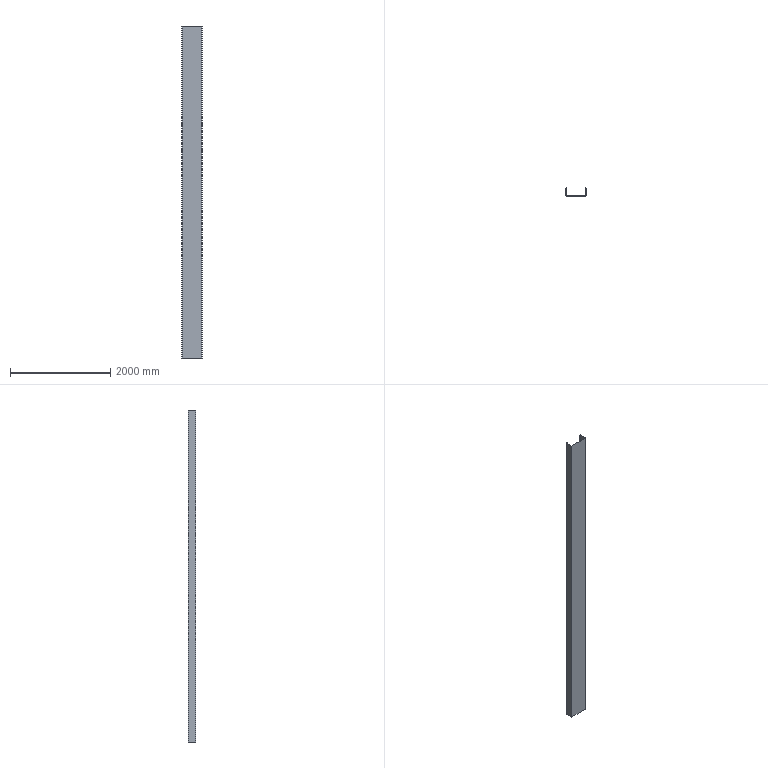Part | STEP file | 750038232 | 1 solid | 22 faces | box 400 x 150 x 6614 mm | volume 7243143 mm3 | plane 14 | cylinder 8 | commonest cylinder face diameters 3 x4 6 x4
STEP:
#1=CARTESIAN_POINT('',(-197.,0.,0.));
#2=VERTEX_POINT('',#1);
#3=CARTESIAN_POINT('',(-197.,0.,6613.5));
#4=VERTEX_POINT('',#3);
#5=CARTESIAN_POINT('',(-197.,0.,0.));
#6=DIRECTION('',(0.,0.,1.));
#7=VECTOR('',#6,1000.);
#8=LINE('',#5,#7);
#9=EDGE_CURVE('',#2,#4,#8,.T.);
#10=ORIENTED_EDGE('',*,*,#9,.F.);
#11=CARTESIAN_POINT('',(197.,0.,0.));
#12=VERTEX_POINT('',#11);
#13=CARTESIAN_POINT('',(200.,0.,0.));
#14=DIRECTION('',(-1.,0.,0.));
#15=VECTOR('',#14,1000.);
#16=LINE('',#13,#15);
#17=EDGE_CURVE('',#12,#2,#16,.T.);
#18=ORIENTED_EDGE('',*,*,#17,.F.);
#19=CARTESIAN_POINT('',(197.,0.,6613.5));
#20=VERTEX_POINT('',#19);
#21=CARTESIAN_POINT('',(197.,0.,0.));
#22=DIRECTION('',(0.,0.,-1.));
#23=VECTOR('',#22,1000.);
#24=LINE('',#21,#23);
#25=EDGE_CURVE('',#20,#12,#24,.T.);
#26=ORIENTED_EDGE('',*,*,#25,.F.);
#27=CARTESIAN_POINT('',(200.,0.,6613.5));
#28=DIRECTION('',(1.,0.,0.));
#29=VECTOR('',#28,1000.);
#30=LINE('',#27,#29);
#31=EDGE_CURVE('',#4,#20,#30,.T.);
#32=ORIENTED_EDGE('',*,*,#31,.F.);
#33=EDGE_LOOP('',(#10,#18,#26,#32));
#34=FACE_OUTER_BOUND('',#33,.T.);
#35=CARTESIAN_POINT('',(200.,0.,0.));
#36=DIRECTION('',(0.,1.,0.));
#37=DIRECTION('',(0.,0.,1.));
#38=AXIS2_PLACEMENT_3D('',#35,#36,#37);
#39=PLANE('',#38);
#40=ADVANCED_FACE('',(#34),#39,.F.);
#41=CARTESIAN_POINT('',(198.5,3.,6613.5));
#42=VERTEX_POINT('',#41);
#43=CARTESIAN_POINT('',(198.5,147.,6613.5));
#44=VERTEX_POINT('',#43);
#45=CARTESIAN_POINT('',(198.5,147.,6613.5));
#46=DIRECTION('',(0.,1.,0.));
#47=VECTOR('',#46,1000.);
#48=LINE('',#45,#47);
#49=EDGE_CURVE('',#42,#44,#48,.T.);
#50=ORIENTED_EDGE('',*,*,#49,.F.);
#51=CARTESIAN_POINT('',(197.,1.5,6613.5));
#52=VERTEX_POINT('',#51);
#53=CARTESIAN_POINT('',(197.,3.,6613.5));
#54=DIRECTION('',(0.,0.,1.));
#55=DIRECTION('',(1.,0.,0.));
#56=AXIS2_PLACEMENT_3D('',#53,#54,#55);
#57=CIRCLE('',#56,1.5);
#58=EDGE_CURVE('',#52,#42,#57,.T.);
#59=ORIENTED_EDGE('',*,*,#58,.F.);
#60=CARTESIAN_POINT('',(-197.,1.5,6613.5));
#61=VERTEX_POINT('',#60);
#62=CARTESIAN_POINT('',(197.,1.5,6613.5));
#63=DIRECTION('',(1.,0.,0.));
#64=VECTOR('',#63,1000.);
#65=LINE('',#62,#64);
#66=EDGE_CURVE('',#61,#52,#65,.T.);
#67=ORIENTED_EDGE('',*,*,#66,.F.);
#68=CARTESIAN_POINT('',(-198.5,3.,6613.5));
#69=VERTEX_POINT('',#68);
#70=CARTESIAN_POINT('',(-197.,3.,6613.5));
#71=DIRECTION('',(0.,0.,1.));
#72=DIRECTION('',(1.,0.,0.));
#73=AXIS2_PLACEMENT_3D('',#70,#71,#72);
#74=CIRCLE('',#73,1.5);
#75=EDGE_CURVE('',#69,#61,#74,.T.);
#76=ORIENTED_EDGE('',*,*,#75,.F.);
#77=CARTESIAN_POINT('',(-198.5,147.,6613.5));
#78=VERTEX_POINT('',#77);
#79=CARTESIAN_POINT('',(-198.5,147.,6613.5));
#80=DIRECTION('',(0.,-1.,0.));
#81=VECTOR('',#80,1000.);
#82=LINE('',#79,#81);
#83=EDGE_CURVE('',#78,#69,#82,.T.);
#84=ORIENTED_EDGE('',*,*,#83,.F.);
#85=CARTESIAN_POINT('',(-197.,148.5,6613.5));
#86=VERTEX_POINT('',#85);
#87=CARTESIAN_POINT('',(-197.,147.,6613.5));
#88=DIRECTION('',(0.,0.,1.));
#89=DIRECTION('',(1.,0.,0.));
#90=AXIS2_PLACEMENT_3D('',#87,#88,#89);
#91=CIRCLE('',#90,1.5);
#92=EDGE_CURVE('',#86,#78,#91,.T.);
#93=ORIENTED_EDGE('',*,*,#92,.F.);
#94=CARTESIAN_POINT('',(-180.,148.5,6613.5));
#95=VERTEX_POINT('',#94);
#96=CARTESIAN_POINT('',(197.,148.5,6613.5));
#97=DIRECTION('',(-1.,0.,0.));
#98=VECTOR('',#97,1000.);
#99=LINE('',#96,#98);
#100=EDGE_CURVE('',#95,#86,#99,.T.);
#101=ORIENTED_EDGE('',*,*,#100,.F.);
#102=CARTESIAN_POINT('',(-180.,150.,6613.5));
#103=VERTEX_POINT('',#102);
#104=CARTESIAN_POINT('',(-180.,150.,6613.5));
#105=DIRECTION('',(0.,-1.,0.));
#106=VECTOR('',#105,1000.);
#107=LINE('',#104,#106);
#108=EDGE_CURVE('',#103,#95,#107,.T.);
#109=ORIENTED_EDGE('',*,*,#108,.F.);
#110=CARTESIAN_POINT('',(-197.,150.,6613.5));
#111=VERTEX_POINT('',#110);
#112=CARTESIAN_POINT('',(197.,150.,6613.5));
#113=DIRECTION('',(1.,0.,0.));
#114=VECTOR('',#113,1000.);
#115=LINE('',#112,#114);
#116=EDGE_CURVE('',#111,#103,#115,.T.);
#117=ORIENTED_EDGE('',*,*,#116,.F.);
#118=CARTESIAN_POINT('',(-200.,147.,6613.5));
#119=VERTEX_POINT('',#118);
#120=CARTESIAN_POINT('',(-197.,147.,6613.5));
#121=DIRECTION('',(0.,0.,-1.));
#122=DIRECTION('',(1.,0.,0.));
#123=AXIS2_PLACEMENT_3D('',#120,#121,#122);
#124=CIRCLE('',#123,3.);
#125=EDGE_CURVE('',#119,#111,#124,.T.);
#126=ORIENTED_EDGE('',*,*,#125,.F.);
#127=CARTESIAN_POINT('',(-200.,3.,6613.5));
#128=VERTEX_POINT('',#127);
#129=CARTESIAN_POINT('',(-200.,147.,6613.5));
#130=DIRECTION('',(0.,1.,0.));
#131=VECTOR('',#130,1000.);
#132=LINE('',#129,#131);
#133=EDGE_CURVE('',#128,#119,#132,.T.);
#134=ORIENTED_EDGE('',*,*,#133,.F.);
#135=CARTESIAN_POINT('',(-197.,3.,6613.5));
#136=DIRECTION('',(0.,0.,-1.));
#137=DIRECTION('',(1.,0.,0.));
#138=AXIS2_PLACEMENT_3D('',#135,#136,#137);
#139=CIRCLE('',#138,3.);
#140=EDGE_CURVE('',#4,#128,#139,.T.);
#141=ORIENTED_EDGE('',*,*,#140,.F.);
#142=ORIENTED_EDGE('',*,*,#31,.T.);
#143=CARTESIAN_POINT('',(200.,3.,6613.5));
#144=VERTEX_POINT('',#143);
#145=CARTESIAN_POINT('',(197.,3.,6613.5));
#146=DIRECTION('',(0.,0.,-1.));
#147=DIRECTION('',(1.,0.,0.));
#148=AXIS2_PLACEMENT_3D('',#145,#146,#147);
#149=CIRCLE('',#148,3.);
#150=EDGE_CURVE('',#144,#20,#149,.T.);
#151=ORIENTED_EDGE('',*,*,#150,.F.);
#152=CARTESIAN_POINT('',(200.,147.,6613.5));
#153=VERTEX_POINT('',#152);
#154=CARTESIAN_POINT('',(200.,147.,6613.5));
#155=DIRECTION('',(0.,-1.,0.));
#156=VECTOR('',#155,1000.);
#157=LINE('',#154,#156);
#158=EDGE_CURVE('',#153,#144,#157,.T.);
#159=ORIENTED_EDGE('',*,*,#158,.F.);
#160=CARTESIAN_POINT('',(197.,150.,6613.5));
#161=VERTEX_POINT('',#160);
#162=CARTESIAN_POINT('',(197.,147.,6613.5));
#163=DIRECTION('',(0.,0.,-1.));
#164=DIRECTION('',(1.,0.,0.));
#165=AXIS2_PLACEMENT_3D('',#162,#163,#164);
#166=CIRCLE('',#165,3.);
#167=EDGE_CURVE('',#161,#153,#166,.T.);
#168=ORIENTED_EDGE('',*,*,#167,.F.);
#169=CARTESIAN_POINT('',(180.,150.,6613.5));
#170=VERTEX_POINT('',#169);
#171=CARTESIAN_POINT('',(197.,150.,6613.5));
#172=DIRECTION('',(1.,0.,0.));
#173=VECTOR('',#172,1000.);
#174=LINE('',#171,#173);
#175=EDGE_CURVE('',#170,#161,#174,.T.);
#176=ORIENTED_EDGE('',*,*,#175,.F.);
#177=CARTESIAN_POINT('',(180.,148.5,6613.5));
#178=VERTEX_POINT('',#177);
#179=CARTESIAN_POINT('',(180.,150.,6613.5));
#180=DIRECTION('',(0.,-1.,0.));
#181=VECTOR('',#180,1000.);
#182=LINE('',#179,#181);
#183=EDGE_CURVE('',#170,#178,#182,.T.);
#184=ORIENTED_EDGE('',*,*,#183,.T.);
#185=CARTESIAN_POINT('',(197.,148.5,6613.5));
#186=VERTEX_POINT('',#185);
#187=CARTESIAN_POINT('',(197.,148.5,6613.5));
#188=DIRECTION('',(-1.,0.,0.));
#189=VECTOR('',#188,1000.);
#190=LINE('',#187,#189);
#191=EDGE_CURVE('',#186,#178,#190,.T.);
#192=ORIENTED_EDGE('',*,*,#191,.F.);
#193=CARTESIAN_POINT('',(197.,147.,6613.5));
#194=DIRECTION('',(0.,0.,1.));
#195=DIRECTION('',(1.,0.,0.));
#196=AXIS2_PLACEMENT_3D('',#193,#194,#195);
#197=CIRCLE('',#196,1.5);
#198=EDGE_CURVE('',#44,#186,#197,.T.);
#199=ORIENTED_EDGE('',*,*,#198,.F.);
#200=EDGE_LOOP('',(#50,#59,#67,#76,#84,#93,#101,#109,#117,#126,#134,#141,#142,#151,#159,#168,#176,#184,#192,#199));
#201=FACE_OUTER_BOUND('',#200,.T.);
#202=CARTESIAN_POINT('',(197.,147.,6613.5));
#203=DIRECTION('',(0.,0.,-1.));
#204=DIRECTION('',(-1.,0.,0.));
#205=AXIS2_PLACEMENT_3D('',#202,#203,#204);
#206=PLANE('',#205);
#207=ADVANCED_FACE('',(#201),#206,.F.);
#208=CARTESIAN_POINT('',(-200.,3.,0.));
#209=VERTEX_POINT('',#208);
#210=CARTESIAN_POINT('',(-197.,3.,0.));
#211=DIRECTION('',(0.,0.,1.));
#212=DIRECTION('',(1.,0.,0.));
#213=AXIS2_PLACEMENT_3D('',#210,#211,#212);
#214=CIRCLE('',#213,3.);
#215=EDGE_CURVE('',#209,#2,#214,.T.);
#216=ORIENTED_EDGE('',*,*,#215,.T.);
#217=ORIENTED_EDGE('',*,*,#9,.T.);
#218=ORIENTED_EDGE('',*,*,#140,.T.);
#219=CARTESIAN_POINT('',(-200.,3.,0.));
#220=DIRECTION('',(0.,0.,-1.));
#221=VECTOR('',#220,1000.);
#222=LINE('',#219,#221);
#223=EDGE_CURVE('',#128,#209,#222,.T.);
#224=ORIENTED_EDGE('',*,*,#223,.T.);
#225=EDGE_LOOP('',(#216,#217,#218,#224));
#226=FACE_OUTER_BOUND('',#225,.T.);
#227=CARTESIAN_POINT('',(-197.,3.,0.));
#228=DIRECTION('',(0.,0.,1.));
#229=DIRECTION('',(1.,0.,0.));
#230=AXIS2_PLACEMENT_3D('',#227,#228,#229);
#231=CYLINDRICAL_SURFACE('',#230,3.);
#232=ADVANCED_FACE('',(#226),#231,.T.);
#233=CARTESIAN_POINT('',(197.,148.5,0.));
#234=VERTEX_POINT('',#233);
#235=CARTESIAN_POINT('',(180.,148.5,0.));
#236=VERTEX_POINT('',#235);
#237=CARTESIAN_POINT('',(180.,148.5,0.));
#238=DIRECTION('',(-1.,0.,0.));
#239=VECTOR('',#238,1000.);
#240=LINE('',#237,#239);
#241=EDGE_CURVE('',#234,#236,#240,.T.);
#242=ORIENTED_EDGE('',*,*,#241,.T.);
#243=CARTESIAN_POINT('',(180.,150.,0.));
#244=VERTEX_POINT('',#243);
#245=CARTESIAN_POINT('',(180.,150.,0.));
#246=DIRECTION('',(0.,1.,0.));
#247=VECTOR('',#246,1000.);
#248=LINE('',#245,#247);
#249=EDGE_CURVE('',#236,#244,#248,.T.);
#250=ORIENTED_EDGE('',*,*,#249,.T.);
#251=CARTESIAN_POINT('',(197.,150.,0.));
#252=VERTEX_POINT('',#251);
#253=CARTESIAN_POINT('',(180.,150.,0.));
#254=DIRECTION('',(1.,0.,0.));
#255=VECTOR('',#254,1000.);
#256=LINE('',#253,#255);
#257=EDGE_CURVE('',#244,#252,#256,.T.);
#258=ORIENTED_EDGE('',*,*,#257,.T.);
#259=CARTESIAN_POINT('',(200.,147.,0.));
#260=VERTEX_POINT('',#259);
#261=CARTESIAN_POINT('',(197.,147.,0.));
#262=DIRECTION('',(0.,0.,-1.));
#263=DIRECTION('',(1.,0.,0.));
#264=AXIS2_PLACEMENT_3D('',#261,#262,#263);
#265=CIRCLE('',#264,3.);
#266=EDGE_CURVE('',#252,#260,#265,.T.);
#267=ORIENTED_EDGE('',*,*,#266,.T.);
#268=CARTESIAN_POINT('',(200.,3.,0.));
#269=VERTEX_POINT('',#268);
#270=CARTESIAN_POINT('',(200.,150.,0.));
#271=DIRECTION('',(0.,-1.,0.));
#272=VECTOR('',#271,1000.);
#273=LINE('',#270,#272);
#274=EDGE_CURVE('',#260,#269,#273,.T.);
#275=ORIENTED_EDGE('',*,*,#274,.T.);
#276=CARTESIAN_POINT('',(197.,3.,0.));
#277=DIRECTION('',(0.,0.,-1.));
#278=DIRECTION('',(1.,0.,0.));
#279=AXIS2_PLACEMENT_3D('',#276,#277,#278);
#280=CIRCLE('',#279,3.);
#281=EDGE_CURVE('',#269,#12,#280,.T.);
#282=ORIENTED_EDGE('',*,*,#281,.T.);
#283=ORIENTED_EDGE('',*,*,#17,.T.);
#284=ORIENTED_EDGE('',*,*,#215,.F.);
#285=CARTESIAN_POINT('',(-200.,147.,0.));
#286=VERTEX_POINT('',#285);
#287=CARTESIAN_POINT('',(-200.,150.,0.));
#288=DIRECTION('',(0.,1.,0.));
#289=VECTOR('',#288,1000.);
#290=LINE('',#287,#289);
#291=EDGE_CURVE('',#209,#286,#290,.T.);
#292=ORIENTED_EDGE('',*,*,#291,.T.);
#293=CARTESIAN_POINT('',(-197.,150.,0.));
#294=VERTEX_POINT('',#293);
#295=CARTESIAN_POINT('',(-197.,147.,0.));
#296=DIRECTION('',(0.,0.,-1.));
#297=DIRECTION('',(1.,0.,0.));
#298=AXIS2_PLACEMENT_3D('',#295,#296,#297);
#299=CIRCLE('',#298,3.);
#300=EDGE_CURVE('',#286,#294,#299,.T.);
#301=ORIENTED_EDGE('',*,*,#300,.T.);
#302=CARTESIAN_POINT('',(-180.,150.,0.));
#303=VERTEX_POINT('',#302);
#304=CARTESIAN_POINT('',(180.,150.,0.));
#305=DIRECTION('',(1.,0.,0.));
#306=VECTOR('',#305,1000.);
#307=LINE('',#304,#306);
#308=EDGE_CURVE('',#294,#303,#307,.T.);
#309=ORIENTED_EDGE('',*,*,#308,.T.);
#310=CARTESIAN_POINT('',(-180.,148.5,0.));
#311=VERTEX_POINT('',#310);
#312=CARTESIAN_POINT('',(-180.,150.,0.));
#313=DIRECTION('',(0.,1.,0.));
#314=VECTOR('',#313,1000.);
#315=LINE('',#312,#314);
#316=EDGE_CURVE('',#311,#303,#315,.T.);
#317=ORIENTED_EDGE('',*,*,#316,.F.);
#318=CARTESIAN_POINT('',(-197.,148.5,0.));
#319=VERTEX_POINT('',#318);
#320=CARTESIAN_POINT('',(180.,148.5,0.));
#321=DIRECTION('',(-1.,0.,0.));
#322=VECTOR('',#321,1000.);
#323=LINE('',#320,#322);
#324=EDGE_CURVE('',#311,#319,#323,.T.);
#325=ORIENTED_EDGE('',*,*,#324,.T.);
#326=CARTESIAN_POINT('',(-198.5,147.,0.));
#327=VERTEX_POINT('',#326);
#328=CARTESIAN_POINT('',(-197.,147.,0.));
#329=DIRECTION('',(0.,0.,1.));
#330=DIRECTION('',(1.,0.,0.));
#331=AXIS2_PLACEMENT_3D('',#328,#329,#330);
#332=CIRCLE('',#331,1.5);
#333=EDGE_CURVE('',#319,#327,#332,.T.);
#334=ORIENTED_EDGE('',*,*,#333,.T.);
#335=CARTESIAN_POINT('',(-198.5,3.,0.));
#336=VERTEX_POINT('',#335);
#337=CARTESIAN_POINT('',(-198.5,150.,0.));
#338=DIRECTION('',(0.,-1.,0.));
#339=VECTOR('',#338,1000.);
#340=LINE('',#337,#339);
#341=EDGE_CURVE('',#327,#336,#340,.T.);
#342=ORIENTED_EDGE('',*,*,#341,.T.);
#343=CARTESIAN_POINT('',(-197.,1.5,0.));
#344=VERTEX_POINT('',#343);
#345=CARTESIAN_POINT('',(-197.,3.,0.));
#346=DIRECTION('',(0.,0.,1.));
#347=DIRECTION('',(1.,0.,0.));
#348=AXIS2_PLACEMENT_3D('',#345,#346,#347);
#349=CIRCLE('',#348,1.5);
#350=EDGE_CURVE('',#336,#344,#349,.T.);
#351=ORIENTED_EDGE('',*,*,#350,.T.);
#352=CARTESIAN_POINT('',(197.,1.5,0.));
#353=VERTEX_POINT('',#352);
#354=CARTESIAN_POINT('',(180.,1.5,0.));
#355=DIRECTION('',(1.,0.,0.));
#356=VECTOR('',#355,1000.);
#357=LINE('',#354,#356);
#358=EDGE_CURVE('',#344,#353,#357,.T.);
#359=ORIENTED_EDGE('',*,*,#358,.T.);
#360=CARTESIAN_POINT('',(198.5,3.,0.));
#361=VERTEX_POINT('',#360);
#362=CARTESIAN_POINT('',(197.,3.,0.));
#363=DIRECTION('',(0.,0.,1.));
#364=DIRECTION('',(1.,0.,0.));
#365=AXIS2_PLACEMENT_3D('',#362,#363,#364);
#366=CIRCLE('',#365,1.5);
#367=EDGE_CURVE('',#353,#361,#366,.T.);
#368=ORIENTED_EDGE('',*,*,#367,.T.);
#369=CARTESIAN_POINT('',(198.5,147.,0.));
#370=VERTEX_POINT('',#369);
#371=CARTESIAN_POINT('',(198.5,150.,0.));
#372=DIRECTION('',(0.,1.,0.));
#373=VECTOR('',#372,1000.);
#374=LINE('',#371,#373);
#375=EDGE_CURVE('',#361,#370,#374,.T.);
#376=ORIENTED_EDGE('',*,*,#375,.T.);
#377=CARTESIAN_POINT('',(197.,147.,0.));
#378=DIRECTION('',(0.,0.,1.));
#379=DIRECTION('',(1.,0.,0.));
#380=AXIS2_PLACEMENT_3D('',#377,#378,#379);
#381=CIRCLE('',#380,1.5);
#382=EDGE_CURVE('',#370,#234,#381,.T.);
#383=ORIENTED_EDGE('',*,*,#382,.T.);
#384=EDGE_LOOP('',(#242,#250,#258,#267,#275,#282,#283,#284,#292,#301,#309,#317,#325,#334,#342,#351,#359,#368,#376,#383));
#385=FACE_OUTER_BOUND('',#384,.T.);
#386=CARTESIAN_POINT('',(180.,150.,0.));
#387=DIRECTION('',(0.,0.,-1.));
#388=DIRECTION('',(-1.,0.,0.));
#389=AXIS2_PLACEMENT_3D('',#386,#387,#388);
#390=PLANE('',#389);
#391=ADVANCED_FACE('',(#385),#390,.T.);
#392=ORIENTED_EDGE('',*,*,#281,.F.);
#393=CARTESIAN_POINT('',(200.,3.,0.));
#394=DIRECTION('',(0.,0.,1.));
#395=VECTOR('',#394,1000.);
#396=LINE('',#393,#395);
#397=EDGE_CURVE('',#269,#144,#396,.T.);
#398=ORIENTED_EDGE('',*,*,#397,.T.);
#399=ORIENTED_EDGE('',*,*,#150,.T.);
#400=ORIENTED_EDGE('',*,*,#25,.T.);
#401=EDGE_LOOP('',(#392,#398,#399,#400));
#402=FACE_OUTER_BOUND('',#401,.T.);
#403=CARTESIAN_POINT('',(197.,3.,0.));
#404=DIRECTION('',(0.,0.,1.));
#405=DIRECTION('',(1.,0.,0.));
#406=AXIS2_PLACEMENT_3D('',#403,#404,#405);
#407=CYLINDRICAL_SURFACE('',#406,3.);
#408=ADVANCED_FACE('',(#402),#407,.T.);
#409=CARTESIAN_POINT('',(197.,148.5,0.));
#410=DIRECTION('',(0.,0.,1.));
#411=VECTOR('',#410,1000.);
#412=LINE('',#409,#411);
#413=EDGE_CURVE('',#234,#186,#412,.T.);
#414=ORIENTED_EDGE('',*,*,#413,.F.);
#415=ORIENTED_EDGE('',*,*,#382,.F.);
#416=CARTESIAN_POINT('',(198.5,147.,0.));
#417=DIRECTION('',(0.,0.,-1.));
#418=VECTOR('',#417,1000.);
#419=LINE('',#416,#418);
#420=EDGE_CURVE('',#44,#370,#419,.T.);
#421=ORIENTED_EDGE('',*,*,#420,.F.);
#422=ORIENTED_EDGE('',*,*,#198,.T.);
#423=EDGE_LOOP('',(#414,#415,#421,#422));
#424=FACE_OUTER_BOUND('',#423,.T.);
#425=CARTESIAN_POINT('',(197.,147.,0.));
#426=DIRECTION('',(0.,0.,1.));
#427=DIRECTION('',(1.,0.,0.));
#428=AXIS2_PLACEMENT_3D('',#425,#426,#427);
#429=CYLINDRICAL_SURFACE('',#428,1.5);
#430=ADVANCED_FACE('',(#424),#429,.F.);
#431=ORIENTED_EDGE('',*,*,#375,.F.);
#432=CARTESIAN_POINT('',(198.5,3.,0.));
#433=DIRECTION('',(0.,0.,1.));
#434=VECTOR('',#433,1000.);
#435=LINE('',#432,#434);
#436=EDGE_CURVE('',#361,#42,#435,.T.);
#437=ORIENTED_EDGE('',*,*,#436,.T.);
#438=ORIENTED_EDGE('',*,*,#49,.T.);
#439=ORIENTED_EDGE('',*,*,#420,.T.);
#440=EDGE_LOOP('',(#431,#437,#438,#439));
#441=FACE_OUTER_BOUND('',#440,.T.);
#442=CARTESIAN_POINT('',(198.5,150.,0.));
#443=DIRECTION('',(-1.,0.,0.));
#444=DIRECTION('',(0.,0.,1.));
#445=AXIS2_PLACEMENT_3D('',#442,#443,#444);
#446=PLANE('',#445);
#447=ADVANCED_FACE('',(#441),#446,.T.);
#448=ORIENTED_EDGE('',*,*,#436,.F.);
#449=ORIENTED_EDGE('',*,*,#367,.F.);
#450=CARTESIAN_POINT('',(197.,1.5,0.));
#451=DIRECTION('',(0.,0.,-1.));
#452=VECTOR('',#451,1000.);
#453=LINE('',#450,#452);
#454=EDGE_CURVE('',#52,#353,#453,.T.);
#455=ORIENTED_EDGE('',*,*,#454,.F.);
#456=ORIENTED_EDGE('',*,*,#58,.T.);
#457=EDGE_LOOP('',(#448,#449,#455,#456));
#458=FACE_OUTER_BOUND('',#457,.T.);
#459=CARTESIAN_POINT('',(197.,3.,0.));
#460=DIRECTION('',(0.,0.,1.));
#461=DIRECTION('',(1.,0.,0.));
#462=AXIS2_PLACEMENT_3D('',#459,#460,#461);
#463=CYLINDRICAL_SURFACE('',#462,1.5);
#464=ADVANCED_FACE('',(#458),#463,.F.);
#465=ORIENTED_EDGE('',*,*,#358,.F.);
#466=CARTESIAN_POINT('',(-197.,1.5,0.));
#467=DIRECTION('',(0.,0.,1.));
#468=VECTOR('',#467,1000.);
#469=LINE('',#466,#468);
#470=EDGE_CURVE('',#344,#61,#469,.T.);
#471=ORIENTED_EDGE('',*,*,#470,.T.);
#472=ORIENTED_EDGE('',*,*,#66,.T.);
#473=ORIENTED_EDGE('',*,*,#454,.T.);
#474=EDGE_LOOP('',(#465,#471,#472,#473));
#475=FACE_OUTER_BOUND('',#474,.T.);
#476=CARTESIAN_POINT('',(200.,1.5,0.));
#477=DIRECTION('',(0.,1.,0.));
#478=DIRECTION('',(0.,0.,1.));
#479=AXIS2_PLACEMENT_3D('',#476,#477,#478);
#480=PLANE('',#479);
#481=ADVANCED_FACE('',(#475),#480,.T.);
#482=ORIENTED_EDGE('',*,*,#470,.F.);
#483=ORIENTED_EDGE('',*,*,#350,.F.);
#484=CARTESIAN_POINT('',(-198.5,3.,0.));
#485=DIRECTION('',(0.,0.,-1.));
#486=VECTOR('',#485,1000.);
#487=LINE('',#484,#486);
#488=EDGE_CURVE('',#69,#336,#487,.T.);
#489=ORIENTED_EDGE('',*,*,#488,.F.);
#490=ORIENTED_EDGE('',*,*,#75,.T.);
#491=EDGE_LOOP('',(#482,#483,#489,#490));
#492=FACE_OUTER_BOUND('',#491,.T.);
#493=CARTESIAN_POINT('',(-197.,3.,0.));
#494=DIRECTION('',(0.,0.,1.));
#495=DIRECTION('',(1.,0.,0.));
#496=AXIS2_PLACEMENT_3D('',#493,#494,#495);
#497=CYLINDRICAL_SURFACE('',#496,1.5);
#498=ADVANCED_FACE('',(#492),#497,.F.);
#499=ORIENTED_EDGE('',*,*,#341,.F.);
#500=CARTESIAN_POINT('',(-198.5,147.,0.));
#501=DIRECTION('',(0.,0.,1.));
#502=VECTOR('',#501,1000.);
#503=LINE('',#500,#502);
#504=EDGE_CURVE('',#327,#78,#503,.T.);
#505=ORIENTED_EDGE('',*,*,#504,.T.);
#506=ORIENTED_EDGE('',*,*,#83,.T.);
#507=ORIENTED_EDGE('',*,*,#488,.T.);
#508=EDGE_LOOP('',(#499,#505,#506,#507));
#509=FACE_OUTER_BOUND('',#508,.T.);
#510=CARTESIAN_POINT('',(-198.5,0.,0.));
#511=DIRECTION('',(1.,0.,0.));
#512=DIRECTION('',(0.,0.,-1.));
#513=AXIS2_PLACEMENT_3D('',#510,#511,#512);
#514=PLANE('',#513);
#515=ADVANCED_FACE('',(#509),#514,.T.);
#516=ORIENTED_EDGE('',*,*,#504,.F.);
#517=ORIENTED_EDGE('',*,*,#333,.F.);
#518=CARTESIAN_POINT('',(-197.,148.5,0.));
#519=DIRECTION('',(0.,0.,-1.));
#520=VECTOR('',#519,1000.);
#521=LINE('',#518,#520);
#522=EDGE_CURVE('',#86,#319,#521,.T.);
#523=ORIENTED_EDGE('',*,*,#522,.F.);
#524=ORIENTED_EDGE('',*,*,#92,.T.);
#525=EDGE_LOOP('',(#516,#517,#523,#524));
#526=FACE_OUTER_BOUND('',#525,.T.);
#527=CARTESIAN_POINT('',(-197.,147.,0.));
#528=DIRECTION('',(0.,0.,1.));
#529=DIRECTION('',(1.,0.,0.));
#530=AXIS2_PLACEMENT_3D('',#527,#528,#529);
#531=CYLINDRICAL_SURFACE('',#530,1.5);
#532=ADVANCED_FACE('',(#526),#531,.F.);
#533=ORIENTED_EDGE('',*,*,#324,.F.);
#534=CARTESIAN_POINT('',(-180.,148.5,0.));
#535=DIRECTION('',(0.,0.,1.));
#536=VECTOR('',#535,1000.);
#537=LINE('',#534,#536);
#538=EDGE_CURVE('',#311,#95,#537,.T.);
#539=ORIENTED_EDGE('',*,*,#538,.T.);
#540=ORIENTED_EDGE('',*,*,#100,.T.);
#541=ORIENTED_EDGE('',*,*,#522,.T.);
#542=EDGE_LOOP('',(#533,#539,#540,#541));
#543=FACE_OUTER_BOUND('',#542,.T.);
#544=CARTESIAN_POINT('',(-200.,148.5,0.));
#545=DIRECTION('',(0.,-1.,0.));
#546=DIRECTION('',(0.,0.,-1.));
#547=AXIS2_PLACEMENT_3D('',#544,#545,#546);
#548=PLANE('',#547);
#549=ADVANCED_FACE('',(#543),#548,.T.);
#550=CARTESIAN_POINT('',(-180.,150.,0.));
#551=DIRECTION('',(0.,0.,1.));
#552=VECTOR('',#551,1000.);
#553=LINE('',#550,#552);
#554=EDGE_CURVE('',#303,#103,#553,.T.);
#555=ORIENTED_EDGE('',*,*,#554,.F.);
#556=ORIENTED_EDGE('',*,*,#308,.F.);
#557=CARTESIAN_POINT('',(-197.,150.,0.));
#558=DIRECTION('',(0.,0.,-1.));
#559=VECTOR('',#558,1000.);
#560=LINE('',#557,#559);
#561=EDGE_CURVE('',#111,#294,#560,.T.);
#562=ORIENTED_EDGE('',*,*,#561,.F.);
#563=ORIENTED_EDGE('',*,*,#116,.T.);
#564=EDGE_LOOP('',(#555,#556,#562,#563));
#565=FACE_OUTER_BOUND('',#564,.T.);
#566=CARTESIAN_POINT('',(-200.,150.,0.));
#567=DIRECTION('',(0.,-1.,0.));
#568=DIRECTION('',(0.,0.,-1.));
#569=AXIS2_PLACEMENT_3D('',#566,#567,#568);
#570=PLANE('',#569);
#571=ADVANCED_FACE('',(#565),#570,.F.);
#572=ORIENTED_EDGE('',*,*,#300,.F.);
#573=CARTESIAN_POINT('',(-200.,147.,0.));
#574=DIRECTION('',(0.,0.,1.));
#575=VECTOR('',#574,1000.);
#576=LINE('',#573,#575);
#577=EDGE_CURVE('',#286,#119,#576,.T.);
#578=ORIENTED_EDGE('',*,*,#577,.T.);
#579=ORIENTED_EDGE('',*,*,#125,.T.);
#580=ORIENTED_EDGE('',*,*,#561,.T.);
#581=EDGE_LOOP('',(#572,#578,#579,#580));
#582=FACE_OUTER_BOUND('',#581,.T.);
#583=CARTESIAN_POINT('',(-197.,147.,0.));
#584=DIRECTION('',(0.,0.,1.));
#585=DIRECTION('',(1.,0.,0.));
#586=AXIS2_PLACEMENT_3D('',#583,#584,#585);
#587=CYLINDRICAL_SURFACE('',#586,3.);
#588=ADVANCED_FACE('',(#582),#587,.T.);
#589=ORIENTED_EDGE('',*,*,#577,.F.);
#590=ORIENTED_EDGE('',*,*,#291,.F.);
#591=ORIENTED_EDGE('',*,*,#223,.F.);
#592=ORIENTED_EDGE('',*,*,#133,.T.);
#593=EDGE_LOOP('',(#589,#590,#591,#592));
#594=FACE_OUTER_BOUND('',#593,.T.);
#595=CARTESIAN_POINT('',(-200.,0.,0.));
#596=DIRECTION('',(1.,0.,0.));
#597=DIRECTION('',(0.,0.,-1.));
#598=AXIS2_PLACEMENT_3D('',#595,#596,#597);
#599=PLANE('',#598);
#600=ADVANCED_FACE('',(#594),#599,.F.);
#601=ORIENTED_EDGE('',*,*,#397,.F.);
#602=ORIENTED_EDGE('',*,*,#274,.F.);
#603=CARTESIAN_POINT('',(200.,147.,0.));
#604=DIRECTION('',(0.,0.,-1.));
#605=VECTOR('',#604,1000.);
#606=LINE('',#603,#605);
#607=EDGE_CURVE('',#153,#260,#606,.T.);
#608=ORIENTED_EDGE('',*,*,#607,.F.);
#609=ORIENTED_EDGE('',*,*,#158,.T.);
#610=EDGE_LOOP('',(#601,#602,#608,#609));
#611=FACE_OUTER_BOUND('',#610,.T.);
#612=CARTESIAN_POINT('',(200.,150.,0.));
#613=DIRECTION('',(-1.,0.,0.));
#614=DIRECTION('',(0.,0.,1.));
#615=AXIS2_PLACEMENT_3D('',#612,#613,#614);
#616=PLANE('',#615);
#617=ADVANCED_FACE('',(#611),#616,.F.);
#618=ORIENTED_EDGE('',*,*,#266,.F.);
#619=CARTESIAN_POINT('',(197.,150.,0.));
#620=DIRECTION('',(0.,0.,1.));
#621=VECTOR('',#620,1000.);
#622=LINE('',#619,#621);
#623=EDGE_CURVE('',#252,#161,#622,.T.);
#624=ORIENTED_EDGE('',*,*,#623,.T.);
#625=ORIENTED_EDGE('',*,*,#167,.T.);
#626=ORIENTED_EDGE('',*,*,#607,.T.);
#627=EDGE_LOOP('',(#618,#624,#625,#626));
#628=FACE_OUTER_BOUND('',#627,.T.);
#629=CARTESIAN_POINT('',(197.,147.,0.));
#630=DIRECTION('',(0.,0.,1.));
#631=DIRECTION('',(1.,0.,0.));
#632=AXIS2_PLACEMENT_3D('',#629,#630,#631);
#633=CYLINDRICAL_SURFACE('',#632,3.);
#634=ADVANCED_FACE('',(#628),#633,.T.);
#635=ORIENTED_EDGE('',*,*,#623,.F.);
#636=ORIENTED_EDGE('',*,*,#257,.F.);
#637=CARTESIAN_POINT('',(180.,150.,0.));
#638=DIRECTION('',(0.,0.,-1.));
#639=VECTOR('',#638,1000.);
#640=LINE('',#637,#639);
#641=EDGE_CURVE('',#170,#244,#640,.T.);
#642=ORIENTED_EDGE('',*,*,#641,.F.);
#643=ORIENTED_EDGE('',*,*,#175,.T.);
#644=EDGE_LOOP('',(#635,#636,#642,#643));
#645=FACE_OUTER_BOUND('',#644,.T.);
#646=CARTESIAN_POINT('',(180.,150.,0.));
#647=DIRECTION('',(0.,-1.,0.));
#648=DIRECTION('',(0.,0.,-1.));
#649=AXIS2_PLACEMENT_3D('',#646,#647,#648);
#650=PLANE('',#649);
#651=ADVANCED_FACE('',(#645),#650,.F.);
#652=ORIENTED_EDGE('',*,*,#241,.F.);
#653=ORIENTED_EDGE('',*,*,#413,.T.);
#654=ORIENTED_EDGE('',*,*,#191,.T.);
#655=CARTESIAN_POINT('',(180.,148.5,0.));
#656=DIRECTION('',(0.,0.,-1.));
#657=VECTOR('',#656,1000.);
#658=LINE('',#655,#657);
#659=EDGE_CURVE('',#178,#236,#658,.T.);
#660=ORIENTED_EDGE('',*,*,#659,.T.);
#661=EDGE_LOOP('',(#652,#653,#654,#660));
#662=FACE_OUTER_BOUND('',#661,.T.);
#663=CARTESIAN_POINT('',(180.,148.5,0.));
#664=DIRECTION('',(0.,-1.,0.));
#665=DIRECTION('',(0.,0.,-1.));
#666=AXIS2_PLACEMENT_3D('',#663,#664,#665);
#667=PLANE('',#666);
#668=ADVANCED_FACE('',(#662),#667,.T.);
#669=ORIENTED_EDGE('',*,*,#316,.T.);
#670=ORIENTED_EDGE('',*,*,#554,.T.);
#671=ORIENTED_EDGE('',*,*,#108,.T.);
#672=ORIENTED_EDGE('',*,*,#538,.F.);
#673=EDGE_LOOP('',(#669,#670,#671,#672));
#674=FACE_OUTER_BOUND('',#673,.T.);
#675=CARTESIAN_POINT('',(-180.,150.,0.));
#676=DIRECTION('',(1.,0.,0.));
#677=DIRECTION('',(0.,0.,-1.));
#678=AXIS2_PLACEMENT_3D('',#675,#676,#677);
#679=PLANE('',#678);
#680=ADVANCED_FACE('',(#674),#679,.T.);
#681=ORIENTED_EDGE('',*,*,#659,.F.);
#682=ORIENTED_EDGE('',*,*,#183,.F.);
#683=ORIENTED_EDGE('',*,*,#641,.T.);
#684=ORIENTED_EDGE('',*,*,#249,.F.);
#685=EDGE_LOOP('',(#681,#682,#683,#684));
#686=FACE_OUTER_BOUND('',#685,.T.);
#687=CARTESIAN_POINT('',(180.,150.,0.));
#688=DIRECTION('',(1.,0.,0.));
#689=DIRECTION('',(0.,0.,-1.));
#690=AXIS2_PLACEMENT_3D('',#687,#688,#689);
#691=PLANE('',#690);
#692=ADVANCED_FACE('',(#686),#691,.F.);
#693=CLOSED_SHELL('',(#40,#207,#232,#391,#408,#430,#447,#464,#481,#498,#515,#532,#549,#571,#588,#600,#617,#634,#651,#668,#680,#692));
#694=MANIFOLD_SOLID_BREP('',#693);
#695=CARTESIAN_POINT('',(0.,0.,0.));
#696=DIRECTION('',(0.,0.,1.));
#697=DIRECTION('',(1.,0.,0.));
#698=AXIS2_PLACEMENT_3D('',#695,#696,#697);
#699=(LENGTH_UNIT()NAMED_UNIT(*)SI_UNIT(.MILLI.,.METRE.));
#700=UNCERTAINTY_MEASURE_WITH_UNIT(LENGTH_MEASURE(0.00001),#699,'','');
#701=(NAMED_UNIT(*)PLANE_ANGLE_UNIT()SI_UNIT($,.RADIAN.));
#702=(NAMED_UNIT(*)SI_UNIT($,.STERADIAN.)SOLID_ANGLE_UNIT());
#703=(GEOMETRIC_REPRESENTATION_CONTEXT(3)GLOBAL_UNCERTAINTY_ASSIGNED_CONTEXT((#700))GLOBAL_UNIT_ASSIGNED_CONTEXT((#699,#701,#702))REPRESENTATION_CONTEXT('',''));
#704=ADVANCED_BREP_SHAPE_REPRESENTATION('',(#694,#698),#703);